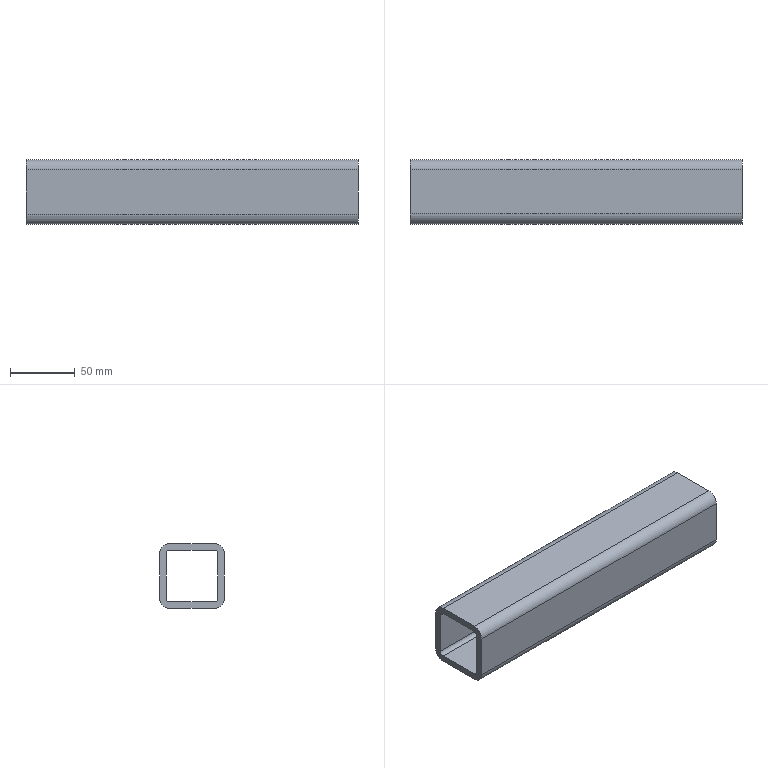Part | SolidWorks | features WeldMemberFeat 1, WeldmentFeature 1 | 1 solid | 18 faces | box 256 x 50 x 50 mm | volume 218314 mm3 | plane 10 | cylinder 8 | commonest cylinder face diameters 6 x4 16 x4
STEP:
#1=CARTESIAN_POINT('',(-88.434,25.,17.));
#2=VERTEX_POINT('',#1);
#3=CARTESIAN_POINT('',(-88.434,17.,25.));
#4=VERTEX_POINT('',#3);
#5=CARTESIAN_POINT('',(-88.434,17.,17.));
#6=DIRECTION('',(1.,0.,0.));
#7=DIRECTION('',(0.,0.,-1.));
#8=AXIS2_PLACEMENT_3D('',#5,#6,#7);
#9=CIRCLE('',#8,8.);
#10=EDGE_CURVE('',#2,#4,#9,.T.);
#11=ORIENTED_EDGE('',*,*,#10,.T.);
#12=CARTESIAN_POINT('',(167.566,17.,25.));
#13=VERTEX_POINT('',#12);
#14=CARTESIAN_POINT('',(167.566,17.,25.));
#15=DIRECTION('',(-1.,0.,0.));
#16=VECTOR('',#15,1000.);
#17=LINE('',#14,#16);
#18=EDGE_CURVE('',#13,#4,#17,.T.);
#19=ORIENTED_EDGE('',*,*,#18,.F.);
#20=CARTESIAN_POINT('',(167.566,25.,17.));
#21=VERTEX_POINT('',#20);
#22=CARTESIAN_POINT('',(167.566,17.,17.));
#23=DIRECTION('',(1.,0.,0.));
#24=DIRECTION('',(0.,0.,-1.));
#25=AXIS2_PLACEMENT_3D('',#22,#23,#24);
#26=CIRCLE('',#25,8.);
#27=EDGE_CURVE('',#21,#13,#26,.T.);
#28=ORIENTED_EDGE('',*,*,#27,.F.);
#29=CARTESIAN_POINT('',(167.566,25.,17.));
#30=DIRECTION('',(-1.,0.,0.));
#31=VECTOR('',#30,1000.);
#32=LINE('',#29,#31);
#33=EDGE_CURVE('',#21,#2,#32,.T.);
#34=ORIENTED_EDGE('',*,*,#33,.T.);
#35=EDGE_LOOP('',(#11,#19,#28,#34));
#36=FACE_OUTER_BOUND('',#35,.T.);
#37=CARTESIAN_POINT('',(167.566,17.,17.));
#38=DIRECTION('',(-1.,0.,0.));
#39=DIRECTION('',(0.,0.,1.));
#40=AXIS2_PLACEMENT_3D('',#37,#38,#39);
#41=CYLINDRICAL_SURFACE('',#40,8.);
#42=ADVANCED_FACE('',(#36),#41,.T.);
#43=CARTESIAN_POINT('',(-88.434,-17.,25.));
#44=VERTEX_POINT('',#43);
#45=CARTESIAN_POINT('',(-88.434,17.,25.));
#46=DIRECTION('',(0.,-1.,0.));
#47=VECTOR('',#46,1000.);
#48=LINE('',#45,#47);
#49=EDGE_CURVE('',#4,#44,#48,.T.);
#50=ORIENTED_EDGE('',*,*,#49,.T.);
#51=CARTESIAN_POINT('',(167.566,-17.,25.));
#52=VERTEX_POINT('',#51);
#53=CARTESIAN_POINT('',(167.566,-17.,25.));
#54=DIRECTION('',(-1.,0.,0.));
#55=VECTOR('',#54,1000.);
#56=LINE('',#53,#55);
#57=EDGE_CURVE('',#52,#44,#56,.T.);
#58=ORIENTED_EDGE('',*,*,#57,.F.);
#59=CARTESIAN_POINT('',(167.566,17.,25.));
#60=DIRECTION('',(0.,-1.,0.));
#61=VECTOR('',#60,1000.);
#62=LINE('',#59,#61);
#63=EDGE_CURVE('',#13,#52,#62,.T.);
#64=ORIENTED_EDGE('',*,*,#63,.F.);
#65=ORIENTED_EDGE('',*,*,#18,.T.);
#66=EDGE_LOOP('',(#50,#58,#64,#65));
#67=FACE_OUTER_BOUND('',#66,.T.);
#68=CARTESIAN_POINT('',(167.566,17.,25.));
#69=DIRECTION('',(0.,0.,-1.));
#70=DIRECTION('',(-1.,0.,0.));
#71=AXIS2_PLACEMENT_3D('',#68,#69,#70);
#72=PLANE('',#71);
#73=ADVANCED_FACE('',(#67),#72,.F.);
#74=CARTESIAN_POINT('',(-88.434,-25.,17.));
#75=VERTEX_POINT('',#74);
#76=CARTESIAN_POINT('',(-88.434,-17.,17.));
#77=DIRECTION('',(1.,0.,0.));
#78=DIRECTION('',(0.,0.,-1.));
#79=AXIS2_PLACEMENT_3D('',#76,#77,#78);
#80=CIRCLE('',#79,8.);
#81=EDGE_CURVE('',#44,#75,#80,.T.);
#82=ORIENTED_EDGE('',*,*,#81,.T.);
#83=CARTESIAN_POINT('',(167.566,-25.,17.));
#84=VERTEX_POINT('',#83);
#85=CARTESIAN_POINT('',(167.566,-25.,17.));
#86=DIRECTION('',(-1.,0.,0.));
#87=VECTOR('',#86,1000.);
#88=LINE('',#85,#87);
#89=EDGE_CURVE('',#84,#75,#88,.T.);
#90=ORIENTED_EDGE('',*,*,#89,.F.);
#91=CARTESIAN_POINT('',(167.566,-17.,17.));
#92=DIRECTION('',(1.,0.,0.));
#93=DIRECTION('',(0.,0.,-1.));
#94=AXIS2_PLACEMENT_3D('',#91,#92,#93);
#95=CIRCLE('',#94,8.);
#96=EDGE_CURVE('',#52,#84,#95,.T.);
#97=ORIENTED_EDGE('',*,*,#96,.F.);
#98=ORIENTED_EDGE('',*,*,#57,.T.);
#99=EDGE_LOOP('',(#82,#90,#97,#98));
#100=FACE_OUTER_BOUND('',#99,.T.);
#101=CARTESIAN_POINT('',(167.566,-17.,17.));
#102=DIRECTION('',(-1.,0.,0.));
#103=DIRECTION('',(0.,0.,1.));
#104=AXIS2_PLACEMENT_3D('',#101,#102,#103);
#105=CYLINDRICAL_SURFACE('',#104,8.);
#106=ADVANCED_FACE('',(#100),#105,.T.);
#107=CARTESIAN_POINT('',(-88.434,-25.,-17.));
#108=VERTEX_POINT('',#107);
#109=CARTESIAN_POINT('',(-88.434,-25.,-17.));
#110=DIRECTION('',(0.,0.,-1.));
#111=VECTOR('',#110,1000.);
#112=LINE('',#109,#111);
#113=EDGE_CURVE('',#75,#108,#112,.T.);
#114=ORIENTED_EDGE('',*,*,#113,.T.);
#115=CARTESIAN_POINT('',(167.566,-25.,-17.));
#116=VERTEX_POINT('',#115);
#117=CARTESIAN_POINT('',(167.566,-25.,-17.));
#118=DIRECTION('',(-1.,0.,0.));
#119=VECTOR('',#118,1000.);
#120=LINE('',#117,#119);
#121=EDGE_CURVE('',#116,#108,#120,.T.);
#122=ORIENTED_EDGE('',*,*,#121,.F.);
#123=CARTESIAN_POINT('',(167.566,-25.,-17.));
#124=DIRECTION('',(0.,0.,-1.));
#125=VECTOR('',#124,1000.);
#126=LINE('',#123,#125);
#127=EDGE_CURVE('',#84,#116,#126,.T.);
#128=ORIENTED_EDGE('',*,*,#127,.F.);
#129=ORIENTED_EDGE('',*,*,#89,.T.);
#130=EDGE_LOOP('',(#114,#122,#128,#129));
#131=FACE_OUTER_BOUND('',#130,.T.);
#132=CARTESIAN_POINT('',(167.566,-25.,-17.));
#133=DIRECTION('',(0.,1.,0.));
#134=DIRECTION('',(0.,0.,1.));
#135=AXIS2_PLACEMENT_3D('',#132,#133,#134);
#136=PLANE('',#135);
#137=ADVANCED_FACE('',(#131),#136,.F.);
#138=CARTESIAN_POINT('',(-88.434,-17.,-25.));
#139=VERTEX_POINT('',#138);
#140=CARTESIAN_POINT('',(-88.434,-17.,-17.));
#141=DIRECTION('',(1.,0.,0.));
#142=DIRECTION('',(0.,0.,-1.));
#143=AXIS2_PLACEMENT_3D('',#140,#141,#142);
#144=CIRCLE('',#143,8.);
#145=EDGE_CURVE('',#108,#139,#144,.T.);
#146=ORIENTED_EDGE('',*,*,#145,.T.);
#147=CARTESIAN_POINT('',(167.566,-17.,-25.));
#148=VERTEX_POINT('',#147);
#149=CARTESIAN_POINT('',(167.566,-17.,-25.));
#150=DIRECTION('',(-1.,0.,0.));
#151=VECTOR('',#150,1000.);
#152=LINE('',#149,#151);
#153=EDGE_CURVE('',#148,#139,#152,.T.);
#154=ORIENTED_EDGE('',*,*,#153,.F.);
#155=CARTESIAN_POINT('',(167.566,-17.,-17.));
#156=DIRECTION('',(1.,0.,0.));
#157=DIRECTION('',(0.,0.,-1.));
#158=AXIS2_PLACEMENT_3D('',#155,#156,#157);
#159=CIRCLE('',#158,8.);
#160=EDGE_CURVE('',#116,#148,#159,.T.);
#161=ORIENTED_EDGE('',*,*,#160,.F.);
#162=ORIENTED_EDGE('',*,*,#121,.T.);
#163=EDGE_LOOP('',(#146,#154,#161,#162));
#164=FACE_OUTER_BOUND('',#163,.T.);
#165=CARTESIAN_POINT('',(167.566,-17.,-17.));
#166=DIRECTION('',(-1.,0.,0.));
#167=DIRECTION('',(0.,0.,1.));
#168=AXIS2_PLACEMENT_3D('',#165,#166,#167);
#169=CYLINDRICAL_SURFACE('',#168,8.);
#170=ADVANCED_FACE('',(#164),#169,.T.);
#171=CARTESIAN_POINT('',(-88.434,17.,-25.));
#172=VERTEX_POINT('',#171);
#173=CARTESIAN_POINT('',(-88.434,-17.,-25.));
#174=DIRECTION('',(0.,1.,0.));
#175=VECTOR('',#174,1000.);
#176=LINE('',#173,#175);
#177=EDGE_CURVE('',#139,#172,#176,.T.);
#178=ORIENTED_EDGE('',*,*,#177,.T.);
#179=CARTESIAN_POINT('',(167.566,17.,-25.));
#180=VERTEX_POINT('',#179);
#181=CARTESIAN_POINT('',(167.566,17.,-25.));
#182=DIRECTION('',(-1.,0.,0.));
#183=VECTOR('',#182,1000.);
#184=LINE('',#181,#183);
#185=EDGE_CURVE('',#180,#172,#184,.T.);
#186=ORIENTED_EDGE('',*,*,#185,.F.);
#187=CARTESIAN_POINT('',(167.566,-17.,-25.));
#188=DIRECTION('',(0.,1.,0.));
#189=VECTOR('',#188,1000.);
#190=LINE('',#187,#189);
#191=EDGE_CURVE('',#148,#180,#190,.T.);
#192=ORIENTED_EDGE('',*,*,#191,.F.);
#193=ORIENTED_EDGE('',*,*,#153,.T.);
#194=EDGE_LOOP('',(#178,#186,#192,#193));
#195=FACE_OUTER_BOUND('',#194,.T.);
#196=CARTESIAN_POINT('',(167.566,-17.,-25.));
#197=DIRECTION('',(0.,0.,1.));
#198=DIRECTION('',(1.,0.,0.));
#199=AXIS2_PLACEMENT_3D('',#196,#197,#198);
#200=PLANE('',#199);
#201=ADVANCED_FACE('',(#195),#200,.F.);
#202=CARTESIAN_POINT('',(-88.434,25.,-17.));
#203=VERTEX_POINT('',#202);
#204=CARTESIAN_POINT('',(-88.434,17.,-17.));
#205=DIRECTION('',(1.,0.,0.));
#206=DIRECTION('',(0.,0.,-1.));
#207=AXIS2_PLACEMENT_3D('',#204,#205,#206);
#208=CIRCLE('',#207,8.);
#209=EDGE_CURVE('',#172,#203,#208,.T.);
#210=ORIENTED_EDGE('',*,*,#209,.T.);
#211=CARTESIAN_POINT('',(167.566,25.,-17.));
#212=VERTEX_POINT('',#211);
#213=CARTESIAN_POINT('',(167.566,25.,-17.));
#214=DIRECTION('',(-1.,0.,0.));
#215=VECTOR('',#214,1000.);
#216=LINE('',#213,#215);
#217=EDGE_CURVE('',#212,#203,#216,.T.);
#218=ORIENTED_EDGE('',*,*,#217,.F.);
#219=CARTESIAN_POINT('',(167.566,17.,-17.));
#220=DIRECTION('',(1.,0.,0.));
#221=DIRECTION('',(0.,0.,-1.));
#222=AXIS2_PLACEMENT_3D('',#219,#220,#221);
#223=CIRCLE('',#222,8.);
#224=EDGE_CURVE('',#180,#212,#223,.T.);
#225=ORIENTED_EDGE('',*,*,#224,.F.);
#226=ORIENTED_EDGE('',*,*,#185,.T.);
#227=EDGE_LOOP('',(#210,#218,#225,#226));
#228=FACE_OUTER_BOUND('',#227,.T.);
#229=CARTESIAN_POINT('',(167.566,17.,-17.));
#230=DIRECTION('',(-1.,0.,0.));
#231=DIRECTION('',(0.,0.,1.));
#232=AXIS2_PLACEMENT_3D('',#229,#230,#231);
#233=CYLINDRICAL_SURFACE('',#232,8.);
#234=ADVANCED_FACE('',(#228),#233,.T.);
#235=CARTESIAN_POINT('',(-88.434,-17.,20.));
#236=VERTEX_POINT('',#235);
#237=CARTESIAN_POINT('',(-88.434,-20.,17.));
#238=VERTEX_POINT('',#237);
#239=CARTESIAN_POINT('',(-88.434,-17.,17.));
#240=DIRECTION('',(1.,0.,0.));
#241=DIRECTION('',(0.,0.,-1.));
#242=AXIS2_PLACEMENT_3D('',#239,#240,#241);
#243=CIRCLE('',#242,3.);
#244=EDGE_CURVE('',#236,#238,#243,.T.);
#245=ORIENTED_EDGE('',*,*,#244,.F.);
#246=CARTESIAN_POINT('',(167.566,-17.,20.));
#247=VERTEX_POINT('',#246);
#248=CARTESIAN_POINT('',(167.566,-17.,20.));
#249=DIRECTION('',(-1.,0.,0.));
#250=VECTOR('',#249,1000.);
#251=LINE('',#248,#250);
#252=EDGE_CURVE('',#247,#236,#251,.T.);
#253=ORIENTED_EDGE('',*,*,#252,.F.);
#254=CARTESIAN_POINT('',(167.566,-20.,17.));
#255=VERTEX_POINT('',#254);
#256=CARTESIAN_POINT('',(167.566,-17.,17.));
#257=DIRECTION('',(1.,0.,0.));
#258=DIRECTION('',(0.,0.,-1.));
#259=AXIS2_PLACEMENT_3D('',#256,#257,#258);
#260=CIRCLE('',#259,3.);
#261=EDGE_CURVE('',#247,#255,#260,.T.);
#262=ORIENTED_EDGE('',*,*,#261,.T.);
#263=CARTESIAN_POINT('',(167.566,-20.,17.));
#264=DIRECTION('',(-1.,0.,0.));
#265=VECTOR('',#264,1000.);
#266=LINE('',#263,#265);
#267=EDGE_CURVE('',#255,#238,#266,.T.);
#268=ORIENTED_EDGE('',*,*,#267,.T.);
#269=EDGE_LOOP('',(#245,#253,#262,#268));
#270=FACE_OUTER_BOUND('',#269,.T.);
#271=CARTESIAN_POINT('',(167.566,-17.,17.));
#272=DIRECTION('',(-1.,0.,0.));
#273=DIRECTION('',(0.,0.,1.));
#274=AXIS2_PLACEMENT_3D('',#271,#272,#273);
#275=CYLINDRICAL_SURFACE('',#274,3.);
#276=ADVANCED_FACE('',(#270),#275,.F.);
#277=CARTESIAN_POINT('',(-88.434,17.,20.));
#278=VERTEX_POINT('',#277);
#279=CARTESIAN_POINT('',(-88.434,17.,20.));
#280=DIRECTION('',(0.,-1.,0.));
#281=VECTOR('',#280,1000.);
#282=LINE('',#279,#281);
#283=EDGE_CURVE('',#278,#236,#282,.T.);
#284=ORIENTED_EDGE('',*,*,#283,.F.);
#285=CARTESIAN_POINT('',(167.566,17.,20.));
#286=VERTEX_POINT('',#285);
#287=CARTESIAN_POINT('',(167.566,17.,20.));
#288=DIRECTION('',(-1.,0.,0.));
#289=VECTOR('',#288,1000.);
#290=LINE('',#287,#289);
#291=EDGE_CURVE('',#286,#278,#290,.T.);
#292=ORIENTED_EDGE('',*,*,#291,.F.);
#293=CARTESIAN_POINT('',(167.566,17.,20.));
#294=DIRECTION('',(0.,-1.,0.));
#295=VECTOR('',#294,1000.);
#296=LINE('',#293,#295);
#297=EDGE_CURVE('',#286,#247,#296,.T.);
#298=ORIENTED_EDGE('',*,*,#297,.T.);
#299=ORIENTED_EDGE('',*,*,#252,.T.);
#300=EDGE_LOOP('',(#284,#292,#298,#299));
#301=FACE_OUTER_BOUND('',#300,.T.);
#302=CARTESIAN_POINT('',(167.566,17.,20.));
#303=DIRECTION('',(0.,0.,-1.));
#304=DIRECTION('',(-1.,0.,0.));
#305=AXIS2_PLACEMENT_3D('',#302,#303,#304);
#306=PLANE('',#305);
#307=ADVANCED_FACE('',(#301),#306,.T.);
#308=CARTESIAN_POINT('',(-88.434,20.,17.));
#309=VERTEX_POINT('',#308);
#310=CARTESIAN_POINT('',(-88.434,17.,17.));
#311=DIRECTION('',(1.,0.,0.));
#312=DIRECTION('',(0.,0.,-1.));
#313=AXIS2_PLACEMENT_3D('',#310,#311,#312);
#314=CIRCLE('',#313,3.);
#315=EDGE_CURVE('',#309,#278,#314,.T.);
#316=ORIENTED_EDGE('',*,*,#315,.F.);
#317=CARTESIAN_POINT('',(167.566,20.,17.));
#318=VERTEX_POINT('',#317);
#319=CARTESIAN_POINT('',(167.566,20.,17.));
#320=DIRECTION('',(-1.,0.,0.));
#321=VECTOR('',#320,1000.);
#322=LINE('',#319,#321);
#323=EDGE_CURVE('',#318,#309,#322,.T.);
#324=ORIENTED_EDGE('',*,*,#323,.F.);
#325=CARTESIAN_POINT('',(167.566,17.,17.));
#326=DIRECTION('',(1.,0.,0.));
#327=DIRECTION('',(0.,0.,-1.));
#328=AXIS2_PLACEMENT_3D('',#325,#326,#327);
#329=CIRCLE('',#328,3.);
#330=EDGE_CURVE('',#318,#286,#329,.T.);
#331=ORIENTED_EDGE('',*,*,#330,.T.);
#332=ORIENTED_EDGE('',*,*,#291,.T.);
#333=EDGE_LOOP('',(#316,#324,#331,#332));
#334=FACE_OUTER_BOUND('',#333,.T.);
#335=CARTESIAN_POINT('',(167.566,17.,17.));
#336=DIRECTION('',(-1.,0.,0.));
#337=DIRECTION('',(0.,0.,1.));
#338=AXIS2_PLACEMENT_3D('',#335,#336,#337);
#339=CYLINDRICAL_SURFACE('',#338,3.);
#340=ADVANCED_FACE('',(#334),#339,.F.);
#341=CARTESIAN_POINT('',(-88.434,20.,-17.));
#342=VERTEX_POINT('',#341);
#343=CARTESIAN_POINT('',(-88.434,20.,17.));
#344=DIRECTION('',(0.,0.,1.));
#345=VECTOR('',#344,1000.);
#346=LINE('',#343,#345);
#347=EDGE_CURVE('',#342,#309,#346,.T.);
#348=ORIENTED_EDGE('',*,*,#347,.F.);
#349=CARTESIAN_POINT('',(167.566,20.,-17.));
#350=VERTEX_POINT('',#349);
#351=CARTESIAN_POINT('',(167.566,20.,-17.));
#352=DIRECTION('',(-1.,0.,0.));
#353=VECTOR('',#352,1000.);
#354=LINE('',#351,#353);
#355=EDGE_CURVE('',#350,#342,#354,.T.);
#356=ORIENTED_EDGE('',*,*,#355,.F.);
#357=CARTESIAN_POINT('',(167.566,20.,17.));
#358=DIRECTION('',(0.,0.,1.));
#359=VECTOR('',#358,1000.);
#360=LINE('',#357,#359);
#361=EDGE_CURVE('',#350,#318,#360,.T.);
#362=ORIENTED_EDGE('',*,*,#361,.T.);
#363=ORIENTED_EDGE('',*,*,#323,.T.);
#364=EDGE_LOOP('',(#348,#356,#362,#363));
#365=FACE_OUTER_BOUND('',#364,.T.);
#366=CARTESIAN_POINT('',(167.566,20.,17.));
#367=DIRECTION('',(0.,-1.,0.));
#368=DIRECTION('',(0.,0.,-1.));
#369=AXIS2_PLACEMENT_3D('',#366,#367,#368);
#370=PLANE('',#369);
#371=ADVANCED_FACE('',(#365),#370,.T.);
#372=CARTESIAN_POINT('',(-88.434,17.,-20.));
#373=VERTEX_POINT('',#372);
#374=CARTESIAN_POINT('',(-88.434,17.,-17.));
#375=DIRECTION('',(1.,0.,0.));
#376=DIRECTION('',(0.,0.,-1.));
#377=AXIS2_PLACEMENT_3D('',#374,#375,#376);
#378=CIRCLE('',#377,3.);
#379=EDGE_CURVE('',#373,#342,#378,.T.);
#380=ORIENTED_EDGE('',*,*,#379,.F.);
#381=CARTESIAN_POINT('',(167.566,17.,-20.));
#382=VERTEX_POINT('',#381);
#383=CARTESIAN_POINT('',(167.566,17.,-20.));
#384=DIRECTION('',(-1.,0.,0.));
#385=VECTOR('',#384,1000.);
#386=LINE('',#383,#385);
#387=EDGE_CURVE('',#382,#373,#386,.T.);
#388=ORIENTED_EDGE('',*,*,#387,.F.);
#389=CARTESIAN_POINT('',(167.566,17.,-17.));
#390=DIRECTION('',(1.,0.,0.));
#391=DIRECTION('',(0.,0.,-1.));
#392=AXIS2_PLACEMENT_3D('',#389,#390,#391);
#393=CIRCLE('',#392,3.);
#394=EDGE_CURVE('',#382,#350,#393,.T.);
#395=ORIENTED_EDGE('',*,*,#394,.T.);
#396=ORIENTED_EDGE('',*,*,#355,.T.);
#397=EDGE_LOOP('',(#380,#388,#395,#396));
#398=FACE_OUTER_BOUND('',#397,.T.);
#399=CARTESIAN_POINT('',(167.566,17.,-17.));
#400=DIRECTION('',(-1.,0.,0.));
#401=DIRECTION('',(0.,0.,1.));
#402=AXIS2_PLACEMENT_3D('',#399,#400,#401);
#403=CYLINDRICAL_SURFACE('',#402,3.);
#404=ADVANCED_FACE('',(#398),#403,.F.);
#405=CARTESIAN_POINT('',(-88.434,-17.,-20.));
#406=VERTEX_POINT('',#405);
#407=CARTESIAN_POINT('',(-88.434,-17.,-20.));
#408=DIRECTION('',(0.,1.,0.));
#409=VECTOR('',#408,1000.);
#410=LINE('',#407,#409);
#411=EDGE_CURVE('',#406,#373,#410,.T.);
#412=ORIENTED_EDGE('',*,*,#411,.F.);
#413=CARTESIAN_POINT('',(167.566,-17.,-20.));
#414=VERTEX_POINT('',#413);
#415=CARTESIAN_POINT('',(167.566,-17.,-20.));
#416=DIRECTION('',(-1.,0.,0.));
#417=VECTOR('',#416,1000.);
#418=LINE('',#415,#417);
#419=EDGE_CURVE('',#414,#406,#418,.T.);
#420=ORIENTED_EDGE('',*,*,#419,.F.);
#421=CARTESIAN_POINT('',(167.566,-17.,-20.));
#422=DIRECTION('',(0.,1.,0.));
#423=VECTOR('',#422,1000.);
#424=LINE('',#421,#423);
#425=EDGE_CURVE('',#414,#382,#424,.T.);
#426=ORIENTED_EDGE('',*,*,#425,.T.);
#427=ORIENTED_EDGE('',*,*,#387,.T.);
#428=EDGE_LOOP('',(#412,#420,#426,#427));
#429=FACE_OUTER_BOUND('',#428,.T.);
#430=CARTESIAN_POINT('',(167.566,-17.,-20.));
#431=DIRECTION('',(0.,0.,1.));
#432=DIRECTION('',(1.,0.,0.));
#433=AXIS2_PLACEMENT_3D('',#430,#431,#432);
#434=PLANE('',#433);
#435=ADVANCED_FACE('',(#429),#434,.T.);
#436=CARTESIAN_POINT('',(-88.434,-20.,-17.));
#437=VERTEX_POINT('',#436);
#438=CARTESIAN_POINT('',(-88.434,-17.,-17.));
#439=DIRECTION('',(1.,0.,0.));
#440=DIRECTION('',(0.,0.,-1.));
#441=AXIS2_PLACEMENT_3D('',#438,#439,#440);
#442=CIRCLE('',#441,3.);
#443=EDGE_CURVE('',#437,#406,#442,.T.);
#444=ORIENTED_EDGE('',*,*,#443,.F.);
#445=CARTESIAN_POINT('',(167.566,-20.,-17.));
#446=VERTEX_POINT('',#445);
#447=CARTESIAN_POINT('',(167.566,-20.,-17.));
#448=DIRECTION('',(-1.,0.,0.));
#449=VECTOR('',#448,1000.);
#450=LINE('',#447,#449);
#451=EDGE_CURVE('',#446,#437,#450,.T.);
#452=ORIENTED_EDGE('',*,*,#451,.F.);
#453=CARTESIAN_POINT('',(167.566,-17.,-17.));
#454=DIRECTION('',(1.,0.,0.));
#455=DIRECTION('',(0.,0.,-1.));
#456=AXIS2_PLACEMENT_3D('',#453,#454,#455);
#457=CIRCLE('',#456,3.);
#458=EDGE_CURVE('',#446,#414,#457,.T.);
#459=ORIENTED_EDGE('',*,*,#458,.T.);
#460=ORIENTED_EDGE('',*,*,#419,.T.);
#461=EDGE_LOOP('',(#444,#452,#459,#460));
#462=FACE_OUTER_BOUND('',#461,.T.);
#463=CARTESIAN_POINT('',(167.566,-17.,-17.));
#464=DIRECTION('',(-1.,0.,0.));
#465=DIRECTION('',(0.,0.,1.));
#466=AXIS2_PLACEMENT_3D('',#463,#464,#465);
#467=CYLINDRICAL_SURFACE('',#466,3.);
#468=ADVANCED_FACE('',(#462),#467,.F.);
#469=CARTESIAN_POINT('',(-88.434,-20.,-17.));
#470=DIRECTION('',(0.,0.,-1.));
#471=VECTOR('',#470,1000.);
#472=LINE('',#469,#471);
#473=EDGE_CURVE('',#238,#437,#472,.T.);
#474=ORIENTED_EDGE('',*,*,#473,.F.);
#475=ORIENTED_EDGE('',*,*,#267,.F.);
#476=CARTESIAN_POINT('',(167.566,-20.,-17.));
#477=DIRECTION('',(0.,0.,-1.));
#478=VECTOR('',#477,1000.);
#479=LINE('',#476,#478);
#480=EDGE_CURVE('',#255,#446,#479,.T.);
#481=ORIENTED_EDGE('',*,*,#480,.T.);
#482=ORIENTED_EDGE('',*,*,#451,.T.);
#483=EDGE_LOOP('',(#474,#475,#481,#482));
#484=FACE_OUTER_BOUND('',#483,.T.);
#485=CARTESIAN_POINT('',(167.566,-20.,-17.));
#486=DIRECTION('',(0.,1.,0.));
#487=DIRECTION('',(0.,0.,1.));
#488=AXIS2_PLACEMENT_3D('',#485,#486,#487);
#489=PLANE('',#488);
#490=ADVANCED_FACE('',(#484),#489,.T.);
#491=CARTESIAN_POINT('',(-88.434,25.,17.));
#492=DIRECTION('',(0.,0.,1.));
#493=VECTOR('',#492,1000.);
#494=LINE('',#491,#493);
#495=EDGE_CURVE('',#203,#2,#494,.T.);
#496=ORIENTED_EDGE('',*,*,#495,.T.);
#497=ORIENTED_EDGE('',*,*,#33,.F.);
#498=CARTESIAN_POINT('',(167.566,25.,17.));
#499=DIRECTION('',(0.,0.,1.));
#500=VECTOR('',#499,1000.);
#501=LINE('',#498,#500);
#502=EDGE_CURVE('',#212,#21,#501,.T.);
#503=ORIENTED_EDGE('',*,*,#502,.F.);
#504=ORIENTED_EDGE('',*,*,#217,.T.);
#505=EDGE_LOOP('',(#496,#497,#503,#504));
#506=FACE_OUTER_BOUND('',#505,.T.);
#507=CARTESIAN_POINT('',(167.566,25.,17.));
#508=DIRECTION('',(0.,-1.,0.));
#509=DIRECTION('',(0.,0.,-1.));
#510=AXIS2_PLACEMENT_3D('',#507,#508,#509);
#511=PLANE('',#510);
#512=ADVANCED_FACE('',(#506),#511,.F.);
#513=ORIENTED_EDGE('',*,*,#261,.F.);
#514=ORIENTED_EDGE('',*,*,#297,.F.);
#515=ORIENTED_EDGE('',*,*,#330,.F.);
#516=ORIENTED_EDGE('',*,*,#361,.F.);
#517=ORIENTED_EDGE('',*,*,#394,.F.);
#518=ORIENTED_EDGE('',*,*,#425,.F.);
#519=ORIENTED_EDGE('',*,*,#458,.F.);
#520=ORIENTED_EDGE('',*,*,#480,.F.);
#521=EDGE_LOOP('',(#513,#514,#515,#516,#517,#518,#519,#520));
#522=FACE_BOUND('',#521,.T.);
#523=ORIENTED_EDGE('',*,*,#27,.T.);
#524=ORIENTED_EDGE('',*,*,#63,.T.);
#525=ORIENTED_EDGE('',*,*,#96,.T.);
#526=ORIENTED_EDGE('',*,*,#127,.T.);
#527=ORIENTED_EDGE('',*,*,#160,.T.);
#528=ORIENTED_EDGE('',*,*,#191,.T.);
#529=ORIENTED_EDGE('',*,*,#224,.T.);
#530=ORIENTED_EDGE('',*,*,#502,.T.);
#531=EDGE_LOOP('',(#523,#524,#525,#526,#527,#528,#529,#530));
#532=FACE_OUTER_BOUND('',#531,.T.);
#533=CARTESIAN_POINT('',(167.566,17.,17.));
#534=DIRECTION('',(1.,0.,0.));
#535=DIRECTION('',(0.,0.,-1.));
#536=AXIS2_PLACEMENT_3D('',#533,#534,#535);
#537=PLANE('',#536);
#538=ADVANCED_FACE('',(#522,#532),#537,.T.);
#539=ORIENTED_EDGE('',*,*,#244,.T.);
#540=ORIENTED_EDGE('',*,*,#473,.T.);
#541=ORIENTED_EDGE('',*,*,#443,.T.);
#542=ORIENTED_EDGE('',*,*,#411,.T.);
#543=ORIENTED_EDGE('',*,*,#379,.T.);
#544=ORIENTED_EDGE('',*,*,#347,.T.);
#545=ORIENTED_EDGE('',*,*,#315,.T.);
#546=ORIENTED_EDGE('',*,*,#283,.T.);
#547=EDGE_LOOP('',(#539,#540,#541,#542,#543,#544,#545,#546));
#548=FACE_BOUND('',#547,.T.);
#549=ORIENTED_EDGE('',*,*,#10,.F.);
#550=ORIENTED_EDGE('',*,*,#495,.F.);
#551=ORIENTED_EDGE('',*,*,#209,.F.);
#552=ORIENTED_EDGE('',*,*,#177,.F.);
#553=ORIENTED_EDGE('',*,*,#145,.F.);
#554=ORIENTED_EDGE('',*,*,#113,.F.);
#555=ORIENTED_EDGE('',*,*,#81,.F.);
#556=ORIENTED_EDGE('',*,*,#49,.F.);
#557=EDGE_LOOP('',(#549,#550,#551,#552,#553,#554,#555,#556));
#558=FACE_OUTER_BOUND('',#557,.T.);
#559=CARTESIAN_POINT('',(-88.434,17.,17.));
#560=DIRECTION('',(1.,0.,0.));
#561=DIRECTION('',(0.,0.,-1.));
#562=AXIS2_PLACEMENT_3D('',#559,#560,#561);
#563=PLANE('',#562);
#564=ADVANCED_FACE('',(#548,#558),#563,.F.);
#565=CLOSED_SHELL('',(#42,#73,#106,#137,#170,#201,#234,#276,#307,#340,#371,#404,#435,#468,#490,#512,#538,#564));
#566=MANIFOLD_SOLID_BREP('',#565);
#567=CARTESIAN_POINT('',(0.,0.,0.));
#568=DIRECTION('',(0.,0.,1.));
#569=DIRECTION('',(1.,0.,0.));
#570=AXIS2_PLACEMENT_3D('',#567,#568,#569);
#571=(LENGTH_UNIT()NAMED_UNIT(*)SI_UNIT(.MILLI.,.METRE.));
#572=UNCERTAINTY_MEASURE_WITH_UNIT(LENGTH_MEASURE(0.00001),#571,'','');
#573=(NAMED_UNIT(*)PLANE_ANGLE_UNIT()SI_UNIT($,.RADIAN.));
#574=(NAMED_UNIT(*)SI_UNIT($,.STERADIAN.)SOLID_ANGLE_UNIT());
#575=(GEOMETRIC_REPRESENTATION_CONTEXT(3)GLOBAL_UNCERTAINTY_ASSIGNED_CONTEXT((#572))GLOBAL_UNIT_ASSIGNED_CONTEXT((#571,#573,#574))REPRESENTATION_CONTEXT('',''));
#576=ADVANCED_BREP_SHAPE_REPRESENTATION('',(#566,#570),#575);